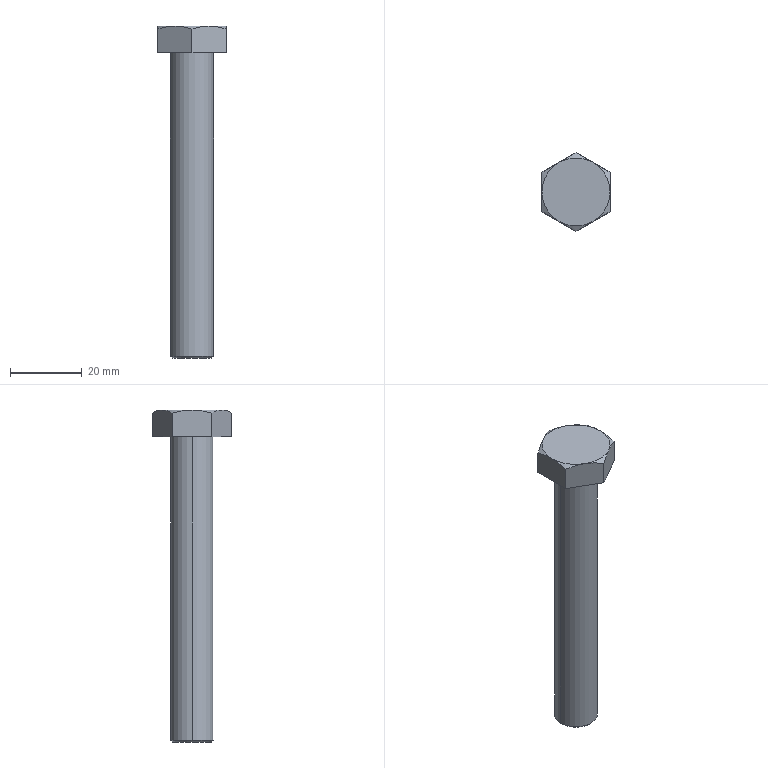Part | STEP file | M12-L85-0 | 1 solid | 19 faces | box 19 x 21.939 x 92.5 mm | volume 11946 mm3 | plane 9 | cone 8 | cylinder 2 | commonest cylinder face diameters 12 x2
STEP:
#1=CARTESIAN_POINT('',(-5.5,0.,-5.));
#2=VERTEX_POINT('',#1);
#3=CARTESIAN_POINT('',(5.5,0.,-5.));
#4=VERTEX_POINT('',#3);
#5=CARTESIAN_POINT('',(0.,0.,-5.));
#6=DIRECTION('',(0.,0.,-1.));
#7=DIRECTION('',(-1.,0.,0.));
#8=AXIS2_PLACEMENT_3D('',#5,#6,#7);
#9=CIRCLE('',#8,5.5);
#10=EDGE_CURVE('',#2,#4,#9,.T.);
#11=ORIENTED_EDGE('',*,*,#10,.F.);
#12=CARTESIAN_POINT('',(-6.,0.,-4.5));
#13=VERTEX_POINT('',#12);
#14=CARTESIAN_POINT('',(-5.5,0.,-5.));
#15=DIRECTION('',(-0.7071,0.,0.7071));
#16=VECTOR('',#15,1000.);
#17=LINE('',#14,#16);
#18=EDGE_CURVE('',#2,#13,#17,.T.);
#19=ORIENTED_EDGE('',*,*,#18,.T.);
#20=CARTESIAN_POINT('',(6.,0.,-4.5));
#21=VERTEX_POINT('',#20);
#22=CARTESIAN_POINT('',(0.,0.,-4.5));
#23=DIRECTION('',(0.,0.,1.));
#24=DIRECTION('',(-1.,0.,0.));
#25=AXIS2_PLACEMENT_3D('',#22,#23,#24);
#26=CIRCLE('',#25,6.);
#27=EDGE_CURVE('',#21,#13,#26,.T.);
#28=ORIENTED_EDGE('',*,*,#27,.F.);
#29=CARTESIAN_POINT('',(5.5,0.,-5.));
#30=DIRECTION('',(0.7071,0.,0.7071));
#31=VECTOR('',#30,1000.);
#32=LINE('',#29,#31);
#33=EDGE_CURVE('',#4,#21,#32,.T.);
#34=ORIENTED_EDGE('',*,*,#33,.F.);
#35=EDGE_LOOP('',(#11,#19,#28,#34));
#36=FACE_OUTER_BOUND('',#35,.T.);
#37=CARTESIAN_POINT('',(0.,0.,-5.));
#38=DIRECTION('',(0.,0.,1.));
#39=DIRECTION('',(1.,0.,0.));
#40=AXIS2_PLACEMENT_3D('',#37,#38,#39);
#41=CONICAL_SURFACE('',#40,5.5,0.7854);
#42=ADVANCED_FACE('',(#36),#41,.T.);
#43=ORIENTED_EDGE('',*,*,#27,.T.);
#44=CARTESIAN_POINT('',(-6.,0.,80.));
#45=VERTEX_POINT('',#44);
#46=CARTESIAN_POINT('',(-6.,0.,0.));
#47=DIRECTION('',(0.,0.,1.));
#48=VECTOR('',#47,1000.);
#49=LINE('',#46,#48);
#50=EDGE_CURVE('',#13,#45,#49,.T.);
#51=ORIENTED_EDGE('',*,*,#50,.T.);
#52=CARTESIAN_POINT('',(6.,0.,80.));
#53=VERTEX_POINT('',#52);
#54=CARTESIAN_POINT('',(0.,0.,80.));
#55=DIRECTION('',(0.,0.,-1.));
#56=DIRECTION('',(1.,0.,0.));
#57=AXIS2_PLACEMENT_3D('',#54,#55,#56);
#58=CIRCLE('',#57,6.);
#59=EDGE_CURVE('',#45,#53,#58,.T.);
#60=ORIENTED_EDGE('',*,*,#59,.T.);
#61=CARTESIAN_POINT('',(6.,0.,0.));
#62=DIRECTION('',(0.,0.,1.));
#63=VECTOR('',#62,1000.);
#64=LINE('',#61,#63);
#65=EDGE_CURVE('',#21,#53,#64,.T.);
#66=ORIENTED_EDGE('',*,*,#65,.F.);
#67=EDGE_LOOP('',(#43,#51,#60,#66));
#68=FACE_OUTER_BOUND('',#67,.T.);
#69=CARTESIAN_POINT('',(0.,0.,0.));
#70=DIRECTION('',(0.,0.,1.));
#71=DIRECTION('',(1.,0.,0.));
#72=AXIS2_PLACEMENT_3D('',#69,#70,#71);
#73=CYLINDRICAL_SURFACE('',#72,6.);
#74=ADVANCED_FACE('',(#68),#73,.T.);
#75=ORIENTED_EDGE('',*,*,#50,.F.);
#76=CARTESIAN_POINT('',(0.,0.,-4.5));
#77=DIRECTION('',(0.,0.,1.));
#78=DIRECTION('',(-1.,0.,0.));
#79=AXIS2_PLACEMENT_3D('',#76,#77,#78);
#80=CIRCLE('',#79,6.);
#81=EDGE_CURVE('',#13,#21,#80,.T.);
#82=ORIENTED_EDGE('',*,*,#81,.T.);
#83=ORIENTED_EDGE('',*,*,#65,.T.);
#84=CARTESIAN_POINT('',(0.,0.,80.));
#85=DIRECTION('',(0.,0.,-1.));
#86=DIRECTION('',(1.,0.,0.));
#87=AXIS2_PLACEMENT_3D('',#84,#85,#86);
#88=CIRCLE('',#87,6.);
#89=EDGE_CURVE('',#53,#45,#88,.T.);
#90=ORIENTED_EDGE('',*,*,#89,.T.);
#91=EDGE_LOOP('',(#75,#82,#83,#90));
#92=FACE_OUTER_BOUND('',#91,.T.);
#93=CARTESIAN_POINT('',(0.,0.,0.));
#94=DIRECTION('',(0.,0.,1.));
#95=DIRECTION('',(1.,0.,0.));
#96=AXIS2_PLACEMENT_3D('',#93,#94,#95);
#97=CYLINDRICAL_SURFACE('',#96,6.);
#98=ADVANCED_FACE('',(#92),#97,.T.);
#99=ORIENTED_EDGE('',*,*,#89,.F.);
#100=ORIENTED_EDGE('',*,*,#59,.F.);
#101=EDGE_LOOP('',(#99,#100));
#102=FACE_BOUND('',#101,.T.);
#103=CARTESIAN_POINT('',(9.5,-5.485,80.));
#104=VERTEX_POINT('',#103);
#105=CARTESIAN_POINT('',(9.5,5.485,80.));
#106=VERTEX_POINT('',#105);
#107=CARTESIAN_POINT('',(9.5,0.,80.));
#108=DIRECTION('',(0.,1.,0.));
#109=VECTOR('',#108,1000.);
#110=LINE('',#107,#109);
#111=EDGE_CURVE('',#104,#106,#110,.T.);
#112=ORIENTED_EDGE('',*,*,#111,.F.);
#113=CARTESIAN_POINT('',(0.,-10.97,80.));
#114=VERTEX_POINT('',#113);
#115=CARTESIAN_POINT('',(0.,-10.97,80.));
#116=DIRECTION('',(0.866,0.5,0.));
#117=VECTOR('',#116,1000.);
#118=LINE('',#115,#117);
#119=EDGE_CURVE('',#114,#104,#118,.T.);
#120=ORIENTED_EDGE('',*,*,#119,.F.);
#121=CARTESIAN_POINT('',(-9.5,-5.485,80.));
#122=VERTEX_POINT('',#121);
#123=CARTESIAN_POINT('',(-9.5,-5.485,80.));
#124=DIRECTION('',(0.866,-0.5,0.));
#125=VECTOR('',#124,1000.);
#126=LINE('',#123,#125);
#127=EDGE_CURVE('',#122,#114,#126,.T.);
#128=ORIENTED_EDGE('',*,*,#127,.F.);
#129=CARTESIAN_POINT('',(-9.5,5.485,80.));
#130=VERTEX_POINT('',#129);
#131=CARTESIAN_POINT('',(-9.5,0.,80.));
#132=DIRECTION('',(0.,-1.,0.));
#133=VECTOR('',#132,1000.);
#134=LINE('',#131,#133);
#135=EDGE_CURVE('',#130,#122,#134,.T.);
#136=ORIENTED_EDGE('',*,*,#135,.F.);
#137=CARTESIAN_POINT('',(0.,10.97,80.));
#138=VERTEX_POINT('',#137);
#139=CARTESIAN_POINT('',(0.,10.97,80.));
#140=DIRECTION('',(-0.866,-0.5,0.));
#141=VECTOR('',#140,1000.);
#142=LINE('',#139,#141);
#143=EDGE_CURVE('',#138,#130,#142,.T.);
#144=ORIENTED_EDGE('',*,*,#143,.F.);
#145=CARTESIAN_POINT('',(9.5,5.485,80.));
#146=DIRECTION('',(-0.866,0.5,0.));
#147=VECTOR('',#146,1000.);
#148=LINE('',#145,#147);
#149=EDGE_CURVE('',#106,#138,#148,.T.);
#150=ORIENTED_EDGE('',*,*,#149,.F.);
#151=EDGE_LOOP('',(#112,#120,#128,#136,#144,#150));
#152=FACE_OUTER_BOUND('',#151,.T.);
#153=CARTESIAN_POINT('',(0.,0.,80.));
#154=DIRECTION('',(0.,0.,1.));
#155=DIRECTION('',(1.,0.,0.));
#156=AXIS2_PLACEMENT_3D('',#153,#154,#155);
#157=PLANE('',#156);
#158=ADVANCED_FACE('',(#102,#152),#157,.F.);
#159=CARTESIAN_POINT('',(0.,10.97,86.651));
#160=VERTEX_POINT('',#159);
#161=CARTESIAN_POINT('',(4.75,8.227,87.5));
#162=VERTEX_POINT('',#161);
#163=CARTESIAN_POINT('',(0.,10.97,86.651));
#164=CARTESIAN_POINT('',(0.776,10.522,86.91));
#165=CARTESIAN_POINT('',(1.558,10.07,87.123));
#166=CARTESIAN_POINT('',(3.14,9.157,87.419));
#167=CARTESIAN_POINT('',(3.939,8.695,87.5));
#168=CARTESIAN_POINT('',(4.75,8.227,87.5));
#169=B_SPLINE_CURVE_WITH_KNOTS('',3,(#163,#164,#165,#166,#167,#168),.UNSPECIFIED.,.F.,.F.,(4,2,4),(0.,0.002775,0.00555),.UNSPECIFIED.);
#170=EDGE_CURVE('',#160,#162,#169,.T.);
#171=ORIENTED_EDGE('',*,*,#170,.T.);
#172=CARTESIAN_POINT('',(9.5,5.485,86.651));
#173=VERTEX_POINT('',#172);
#174=CARTESIAN_POINT('',(4.75,8.227,87.5));
#175=CARTESIAN_POINT('',(5.561,7.759,87.5));
#176=CARTESIAN_POINT('',(6.36,7.298,87.419));
#177=CARTESIAN_POINT('',(7.942,6.384,87.123));
#178=CARTESIAN_POINT('',(8.724,5.933,86.91));
#179=CARTESIAN_POINT('',(9.5,5.485,86.651));
#180=B_SPLINE_CURVE_WITH_KNOTS('',3,(#174,#175,#176,#177,#178,#179),.UNSPECIFIED.,.F.,.F.,(4,2,4),(0.,0.002775,0.00555),.UNSPECIFIED.);
#181=EDGE_CURVE('',#162,#173,#180,.T.);
#182=ORIENTED_EDGE('',*,*,#181,.T.);
#183=CARTESIAN_POINT('',(9.5,5.485,80.));
#184=DIRECTION('',(0.,0.,-1.));
#185=VECTOR('',#184,1000.);
#186=LINE('',#183,#185);
#187=EDGE_CURVE('',#173,#106,#186,.T.);
#188=ORIENTED_EDGE('',*,*,#187,.T.);
#189=ORIENTED_EDGE('',*,*,#149,.T.);
#190=CARTESIAN_POINT('',(0.,10.97,80.));
#191=DIRECTION('',(0.,0.,1.));
#192=VECTOR('',#191,1000.);
#193=LINE('',#190,#192);
#194=EDGE_CURVE('',#138,#160,#193,.T.);
#195=ORIENTED_EDGE('',*,*,#194,.T.);
#196=EDGE_LOOP('',(#171,#182,#188,#189,#195));
#197=FACE_OUTER_BOUND('',#196,.T.);
#198=CARTESIAN_POINT('',(9.5,5.485,80.));
#199=DIRECTION('',(0.5,0.866,0.));
#200=DIRECTION('',(-0.866,0.5,0.));
#201=AXIS2_PLACEMENT_3D('',#198,#199,#200);
#202=PLANE('',#201);
#203=ADVANCED_FACE('',(#197),#202,.T.);
#204=CARTESIAN_POINT('',(9.5,-0.000000001,87.5));
#205=VERTEX_POINT('',#204);
#206=CARTESIAN_POINT('',(9.5,5.485,86.651));
#207=CARTESIAN_POINT('',(9.5,4.589,86.91));
#208=CARTESIAN_POINT('',(9.5,3.686,87.123));
#209=CARTESIAN_POINT('',(9.5,1.859,87.419));
#210=CARTESIAN_POINT('',(9.5,0.936,87.5));
#211=CARTESIAN_POINT('',(9.5,-0.000000001,87.5));
#212=B_SPLINE_CURVE_WITH_KNOTS('',3,(#206,#207,#208,#209,#210,#211),.UNSPECIFIED.,.F.,.F.,(4,2,4),(0.,0.002775,0.00555),.UNSPECIFIED.);
#213=EDGE_CURVE('',#173,#205,#212,.T.);
#214=ORIENTED_EDGE('',*,*,#213,.T.);
#215=CARTESIAN_POINT('',(9.5,-5.485,86.651));
#216=VERTEX_POINT('',#215);
#217=CARTESIAN_POINT('',(9.5,-0.000000001,87.5));
#218=CARTESIAN_POINT('',(9.5,-0.936,87.5));
#219=CARTESIAN_POINT('',(9.5,-1.859,87.419));
#220=CARTESIAN_POINT('',(9.5,-3.686,87.123));
#221=CARTESIAN_POINT('',(9.5,-4.589,86.91));
#222=CARTESIAN_POINT('',(9.5,-5.485,86.651));
#223=B_SPLINE_CURVE_WITH_KNOTS('',3,(#217,#218,#219,#220,#221,#222),.UNSPECIFIED.,.F.,.F.,(4,2,4),(0.,0.002775,0.00555),.UNSPECIFIED.);
#224=EDGE_CURVE('',#205,#216,#223,.T.);
#225=ORIENTED_EDGE('',*,*,#224,.T.);
#226=CARTESIAN_POINT('',(9.5,-5.485,80.));
#227=DIRECTION('',(0.,0.,-1.));
#228=VECTOR('',#227,1000.);
#229=LINE('',#226,#228);
#230=EDGE_CURVE('',#216,#104,#229,.T.);
#231=ORIENTED_EDGE('',*,*,#230,.T.);
#232=ORIENTED_EDGE('',*,*,#111,.T.);
#233=ORIENTED_EDGE('',*,*,#187,.F.);
#234=EDGE_LOOP('',(#214,#225,#231,#232,#233));
#235=FACE_OUTER_BOUND('',#234,.T.);
#236=CARTESIAN_POINT('',(9.5,-5.485,80.));
#237=DIRECTION('',(1.,0.,0.));
#238=DIRECTION('',(0.,0.,-1.));
#239=AXIS2_PLACEMENT_3D('',#236,#237,#238);
#240=PLANE('',#239);
#241=ADVANCED_FACE('',(#235),#240,.T.);
#242=CARTESIAN_POINT('',(4.75,-8.227,87.5));
#243=VERTEX_POINT('',#242);
#244=CARTESIAN_POINT('',(9.5,-5.485,86.651));
#245=CARTESIAN_POINT('',(8.724,-5.933,86.91));
#246=CARTESIAN_POINT('',(7.942,-6.384,87.123));
#247=CARTESIAN_POINT('',(6.36,-7.298,87.419));
#248=CARTESIAN_POINT('',(5.561,-7.759,87.5));
#249=CARTESIAN_POINT('',(4.75,-8.227,87.5));
#250=B_SPLINE_CURVE_WITH_KNOTS('',3,(#244,#245,#246,#247,#248,#249),.UNSPECIFIED.,.F.,.F.,(4,2,4),(0.,0.002775,0.00555),.UNSPECIFIED.);
#251=EDGE_CURVE('',#216,#243,#250,.T.);
#252=ORIENTED_EDGE('',*,*,#251,.T.);
#253=CARTESIAN_POINT('',(0.,-10.97,86.651));
#254=VERTEX_POINT('',#253);
#255=CARTESIAN_POINT('',(4.75,-8.227,87.5));
#256=CARTESIAN_POINT('',(3.939,-8.695,87.5));
#257=CARTESIAN_POINT('',(3.14,-9.157,87.419));
#258=CARTESIAN_POINT('',(1.558,-10.07,87.123));
#259=CARTESIAN_POINT('',(0.776,-10.522,86.91));
#260=CARTESIAN_POINT('',(0.,-10.97,86.651));
#261=B_SPLINE_CURVE_WITH_KNOTS('',3,(#255,#256,#257,#258,#259,#260),.UNSPECIFIED.,.F.,.F.,(4,2,4),(0.,0.002775,0.00555),.UNSPECIFIED.);
#262=EDGE_CURVE('',#243,#254,#261,.T.);
#263=ORIENTED_EDGE('',*,*,#262,.T.);
#264=CARTESIAN_POINT('',(0.,-10.97,80.));
#265=DIRECTION('',(0.,0.,-1.));
#266=VECTOR('',#265,1000.);
#267=LINE('',#264,#266);
#268=EDGE_CURVE('',#254,#114,#267,.T.);
#269=ORIENTED_EDGE('',*,*,#268,.T.);
#270=ORIENTED_EDGE('',*,*,#119,.T.);
#271=ORIENTED_EDGE('',*,*,#230,.F.);
#272=EDGE_LOOP('',(#252,#263,#269,#270,#271));
#273=FACE_OUTER_BOUND('',#272,.T.);
#274=CARTESIAN_POINT('',(0.,-10.97,80.));
#275=DIRECTION('',(0.5,-0.866,0.));
#276=DIRECTION('',(0.866,0.5,0.));
#277=AXIS2_PLACEMENT_3D('',#274,#275,#276);
#278=PLANE('',#277);
#279=ADVANCED_FACE('',(#273),#278,.T.);
#280=CARTESIAN_POINT('',(-4.75,-8.227,87.5));
#281=VERTEX_POINT('',#280);
#282=CARTESIAN_POINT('',(0.,-10.97,86.651));
#283=CARTESIAN_POINT('',(-0.776,-10.522,86.91));
#284=CARTESIAN_POINT('',(-1.558,-10.07,87.123));
#285=CARTESIAN_POINT('',(-3.14,-9.157,87.419));
#286=CARTESIAN_POINT('',(-3.939,-8.695,87.5));
#287=CARTESIAN_POINT('',(-4.75,-8.227,87.5));
#288=B_SPLINE_CURVE_WITH_KNOTS('',3,(#282,#283,#284,#285,#286,#287),.UNSPECIFIED.,.F.,.F.,(4,2,4),(0.,0.002775,0.00555),.UNSPECIFIED.);
#289=EDGE_CURVE('',#254,#281,#288,.T.);
#290=ORIENTED_EDGE('',*,*,#289,.T.);
#291=CARTESIAN_POINT('',(-9.5,-5.485,86.651));
#292=VERTEX_POINT('',#291);
#293=CARTESIAN_POINT('',(-4.75,-8.227,87.5));
#294=CARTESIAN_POINT('',(-5.561,-7.759,87.5));
#295=CARTESIAN_POINT('',(-6.36,-7.298,87.419));
#296=CARTESIAN_POINT('',(-7.942,-6.384,87.123));
#297=CARTESIAN_POINT('',(-8.724,-5.933,86.91));
#298=CARTESIAN_POINT('',(-9.5,-5.485,86.651));
#299=B_SPLINE_CURVE_WITH_KNOTS('',3,(#293,#294,#295,#296,#297,#298),.UNSPECIFIED.,.F.,.F.,(4,2,4),(0.,0.002775,0.00555),.UNSPECIFIED.);
#300=EDGE_CURVE('',#281,#292,#299,.T.);
#301=ORIENTED_EDGE('',*,*,#300,.T.);
#302=CARTESIAN_POINT('',(-9.5,-5.485,80.));
#303=DIRECTION('',(0.,0.,-1.));
#304=VECTOR('',#303,1000.);
#305=LINE('',#302,#304);
#306=EDGE_CURVE('',#292,#122,#305,.T.);
#307=ORIENTED_EDGE('',*,*,#306,.T.);
#308=ORIENTED_EDGE('',*,*,#127,.T.);
#309=ORIENTED_EDGE('',*,*,#268,.F.);
#310=EDGE_LOOP('',(#290,#301,#307,#308,#309));
#311=FACE_OUTER_BOUND('',#310,.T.);
#312=CARTESIAN_POINT('',(-9.5,-5.485,80.));
#313=DIRECTION('',(-0.5,-0.866,0.));
#314=DIRECTION('',(0.866,-0.5,0.));
#315=AXIS2_PLACEMENT_3D('',#312,#313,#314);
#316=PLANE('',#315);
#317=ADVANCED_FACE('',(#311),#316,.T.);
#318=CARTESIAN_POINT('',(-9.5,0.,87.5));
#319=VERTEX_POINT('',#318);
#320=CARTESIAN_POINT('',(-9.5,-5.485,86.651));
#321=CARTESIAN_POINT('',(-9.5,-4.589,86.91));
#322=CARTESIAN_POINT('',(-9.5,-3.686,87.123));
#323=CARTESIAN_POINT('',(-9.5,-1.859,87.419));
#324=CARTESIAN_POINT('',(-9.5,-0.936,87.5));
#325=CARTESIAN_POINT('',(-9.5,0.,87.5));
#326=B_SPLINE_CURVE_WITH_KNOTS('',3,(#320,#321,#322,#323,#324,#325),.UNSPECIFIED.,.F.,.F.,(4,2,4),(0.,0.002775,0.00555),.UNSPECIFIED.);
#327=EDGE_CURVE('',#292,#319,#326,.T.);
#328=ORIENTED_EDGE('',*,*,#327,.T.);
#329=CARTESIAN_POINT('',(-9.5,5.485,86.651));
#330=VERTEX_POINT('',#329);
#331=CARTESIAN_POINT('',(-9.5,0.,87.5));
#332=CARTESIAN_POINT('',(-9.5,0.936,87.5));
#333=CARTESIAN_POINT('',(-9.5,1.859,87.419));
#334=CARTESIAN_POINT('',(-9.5,3.686,87.123));
#335=CARTESIAN_POINT('',(-9.5,4.589,86.91));
#336=CARTESIAN_POINT('',(-9.5,5.485,86.651));
#337=B_SPLINE_CURVE_WITH_KNOTS('',3,(#331,#332,#333,#334,#335,#336),.UNSPECIFIED.,.F.,.F.,(4,2,4),(0.,0.002775,0.00555),.UNSPECIFIED.);
#338=EDGE_CURVE('',#319,#330,#337,.T.);
#339=ORIENTED_EDGE('',*,*,#338,.T.);
#340=CARTESIAN_POINT('',(-9.5,5.485,80.));
#341=DIRECTION('',(0.,0.,-1.));
#342=VECTOR('',#341,1000.);
#343=LINE('',#340,#342);
#344=EDGE_CURVE('',#330,#130,#343,.T.);
#345=ORIENTED_EDGE('',*,*,#344,.T.);
#346=ORIENTED_EDGE('',*,*,#135,.T.);
#347=ORIENTED_EDGE('',*,*,#306,.F.);
#348=EDGE_LOOP('',(#328,#339,#345,#346,#347));
#349=FACE_OUTER_BOUND('',#348,.T.);
#350=CARTESIAN_POINT('',(-9.5,5.485,80.));
#351=DIRECTION('',(-1.,0.,0.));
#352=DIRECTION('',(0.,0.,1.));
#353=AXIS2_PLACEMENT_3D('',#350,#351,#352);
#354=PLANE('',#353);
#355=ADVANCED_FACE('',(#349),#354,.T.);
#356=CARTESIAN_POINT('',(-4.75,8.227,87.5));
#357=VERTEX_POINT('',#356);
#358=CARTESIAN_POINT('',(-9.5,5.485,86.651));
#359=CARTESIAN_POINT('',(-8.724,5.933,86.91));
#360=CARTESIAN_POINT('',(-7.942,6.384,87.123));
#361=CARTESIAN_POINT('',(-6.36,7.298,87.419));
#362=CARTESIAN_POINT('',(-5.561,7.759,87.5));
#363=CARTESIAN_POINT('',(-4.75,8.227,87.5));
#364=B_SPLINE_CURVE_WITH_KNOTS('',3,(#358,#359,#360,#361,#362,#363),.UNSPECIFIED.,.F.,.F.,(4,2,4),(0.,0.002775,0.00555),.UNSPECIFIED.);
#365=EDGE_CURVE('',#330,#357,#364,.T.);
#366=ORIENTED_EDGE('',*,*,#365,.T.);
#367=CARTESIAN_POINT('',(-4.75,8.227,87.5));
#368=CARTESIAN_POINT('',(-3.939,8.695,87.5));
#369=CARTESIAN_POINT('',(-3.14,9.157,87.419));
#370=CARTESIAN_POINT('',(-1.558,10.07,87.123));
#371=CARTESIAN_POINT('',(-0.776,10.522,86.91));
#372=CARTESIAN_POINT('',(0.,10.97,86.651));
#373=B_SPLINE_CURVE_WITH_KNOTS('',3,(#367,#368,#369,#370,#371,#372),.UNSPECIFIED.,.F.,.F.,(4,2,4),(0.,0.002775,0.00555),.UNSPECIFIED.);
#374=EDGE_CURVE('',#357,#160,#373,.T.);
#375=ORIENTED_EDGE('',*,*,#374,.T.);
#376=ORIENTED_EDGE('',*,*,#194,.F.);
#377=ORIENTED_EDGE('',*,*,#143,.T.);
#378=ORIENTED_EDGE('',*,*,#344,.F.);
#379=EDGE_LOOP('',(#366,#375,#376,#377,#378));
#380=FACE_OUTER_BOUND('',#379,.T.);
#381=CARTESIAN_POINT('',(0.,10.97,80.));
#382=DIRECTION('',(-0.5,0.866,0.));
#383=DIRECTION('',(-0.866,-0.5,0.));
#384=AXIS2_PLACEMENT_3D('',#381,#382,#383);
#385=PLANE('',#384);
#386=ADVANCED_FACE('',(#380),#385,.T.);
#387=ORIENTED_EDGE('',*,*,#181,.F.);
#388=CARTESIAN_POINT('',(0.,0.,87.5));
#389=DIRECTION('',(0.,0.,-1.));
#390=DIRECTION('',(-1.,0.,0.));
#391=AXIS2_PLACEMENT_3D('',#388,#389,#390);
#392=CIRCLE('',#391,9.5);
#393=EDGE_CURVE('',#162,#205,#392,.T.);
#394=ORIENTED_EDGE('',*,*,#393,.T.);
#395=ORIENTED_EDGE('',*,*,#213,.F.);
#396=EDGE_LOOP('',(#387,#394,#395));
#397=FACE_OUTER_BOUND('',#396,.T.);
#398=CARTESIAN_POINT('',(0.,0.,86.646));
#399=DIRECTION('',(0.,0.,-1.));
#400=DIRECTION('',(-1.,0.,0.));
#401=AXIS2_PLACEMENT_3D('',#398,#399,#400);
#402=CONICAL_SURFACE('',#401,10.978,1.047);
#403=ADVANCED_FACE('',(#397),#402,.T.);
#404=ORIENTED_EDGE('',*,*,#374,.F.);
#405=CARTESIAN_POINT('',(0.,0.,87.5));
#406=DIRECTION('',(0.,0.,-1.));
#407=DIRECTION('',(-1.,0.,0.));
#408=AXIS2_PLACEMENT_3D('',#405,#406,#407);
#409=CIRCLE('',#408,9.5);
#410=EDGE_CURVE('',#357,#162,#409,.T.);
#411=ORIENTED_EDGE('',*,*,#410,.T.);
#412=ORIENTED_EDGE('',*,*,#170,.F.);
#413=EDGE_LOOP('',(#404,#411,#412));
#414=FACE_OUTER_BOUND('',#413,.T.);
#415=CARTESIAN_POINT('',(0.,0.,86.646));
#416=DIRECTION('',(0.,0.,-1.));
#417=DIRECTION('',(-1.,0.,0.));
#418=AXIS2_PLACEMENT_3D('',#415,#416,#417);
#419=CONICAL_SURFACE('',#418,10.978,1.047);
#420=ADVANCED_FACE('',(#414),#419,.T.);
#421=ORIENTED_EDGE('',*,*,#224,.F.);
#422=CARTESIAN_POINT('',(0.,0.,87.5));
#423=DIRECTION('',(0.,0.,-1.));
#424=DIRECTION('',(-1.,0.,0.));
#425=AXIS2_PLACEMENT_3D('',#422,#423,#424);
#426=CIRCLE('',#425,9.5);
#427=EDGE_CURVE('',#205,#243,#426,.T.);
#428=ORIENTED_EDGE('',*,*,#427,.T.);
#429=ORIENTED_EDGE('',*,*,#251,.F.);
#430=EDGE_LOOP('',(#421,#428,#429));
#431=FACE_OUTER_BOUND('',#430,.T.);
#432=CARTESIAN_POINT('',(0.,0.,86.646));
#433=DIRECTION('',(0.,0.,-1.));
#434=DIRECTION('',(-1.,0.,0.));
#435=AXIS2_PLACEMENT_3D('',#432,#433,#434);
#436=CONICAL_SURFACE('',#435,10.978,1.047);
#437=ADVANCED_FACE('',(#431),#436,.T.);
#438=ORIENTED_EDGE('',*,*,#262,.F.);
#439=CARTESIAN_POINT('',(0.,0.,87.5));
#440=DIRECTION('',(0.,0.,-1.));
#441=DIRECTION('',(-1.,0.,0.));
#442=AXIS2_PLACEMENT_3D('',#439,#440,#441);
#443=CIRCLE('',#442,9.5);
#444=EDGE_CURVE('',#243,#281,#443,.T.);
#445=ORIENTED_EDGE('',*,*,#444,.T.);
#446=ORIENTED_EDGE('',*,*,#289,.F.);
#447=EDGE_LOOP('',(#438,#445,#446));
#448=FACE_OUTER_BOUND('',#447,.T.);
#449=CARTESIAN_POINT('',(0.,0.,86.646));
#450=DIRECTION('',(0.,0.,-1.));
#451=DIRECTION('',(-1.,0.,0.));
#452=AXIS2_PLACEMENT_3D('',#449,#450,#451);
#453=CONICAL_SURFACE('',#452,10.978,1.047);
#454=ADVANCED_FACE('',(#448),#453,.T.);
#455=ORIENTED_EDGE('',*,*,#300,.F.);
#456=CARTESIAN_POINT('',(0.,0.,87.5));
#457=DIRECTION('',(0.,0.,-1.));
#458=DIRECTION('',(-1.,0.,0.));
#459=AXIS2_PLACEMENT_3D('',#456,#457,#458);
#460=CIRCLE('',#459,9.5);
#461=EDGE_CURVE('',#281,#319,#460,.T.);
#462=ORIENTED_EDGE('',*,*,#461,.T.);
#463=ORIENTED_EDGE('',*,*,#327,.F.);
#464=EDGE_LOOP('',(#455,#462,#463));
#465=FACE_OUTER_BOUND('',#464,.T.);
#466=CARTESIAN_POINT('',(0.,0.,86.646));
#467=DIRECTION('',(0.,0.,-1.));
#468=DIRECTION('',(-1.,0.,0.));
#469=AXIS2_PLACEMENT_3D('',#466,#467,#468);
#470=CONICAL_SURFACE('',#469,10.978,1.047);
#471=ADVANCED_FACE('',(#465),#470,.T.);
#472=ORIENTED_EDGE('',*,*,#338,.F.);
#473=CARTESIAN_POINT('',(0.,0.,87.5));
#474=DIRECTION('',(0.,0.,-1.));
#475=DIRECTION('',(-1.,0.,0.));
#476=AXIS2_PLACEMENT_3D('',#473,#474,#475);
#477=CIRCLE('',#476,9.5);
#478=EDGE_CURVE('',#319,#357,#477,.T.);
#479=ORIENTED_EDGE('',*,*,#478,.T.);
#480=ORIENTED_EDGE('',*,*,#365,.F.);
#481=EDGE_LOOP('',(#472,#479,#480));
#482=FACE_OUTER_BOUND('',#481,.T.);
#483=CARTESIAN_POINT('',(0.,0.,86.646));
#484=DIRECTION('',(0.,0.,-1.));
#485=DIRECTION('',(-1.,0.,0.));
#486=AXIS2_PLACEMENT_3D('',#483,#484,#485);
#487=CONICAL_SURFACE('',#486,10.978,1.047);
#488=ADVANCED_FACE('',(#482),#487,.T.);
#489=ORIENTED_EDGE('',*,*,#461,.F.);
#490=ORIENTED_EDGE('',*,*,#444,.F.);
#491=ORIENTED_EDGE('',*,*,#427,.F.);
#492=ORIENTED_EDGE('',*,*,#393,.F.);
#493=ORIENTED_EDGE('',*,*,#410,.F.);
#494=ORIENTED_EDGE('',*,*,#478,.F.);
#495=EDGE_LOOP('',(#489,#490,#491,#492,#493,#494));
#496=FACE_OUTER_BOUND('',#495,.T.);
#497=CARTESIAN_POINT('',(0.,0.,87.5));
#498=DIRECTION('',(0.,0.,1.));
#499=DIRECTION('',(1.,0.,0.));
#500=AXIS2_PLACEMENT_3D('',#497,#498,#499);
#501=PLANE('',#500);
#502=ADVANCED_FACE('',(#496),#501,.T.);
#503=CARTESIAN_POINT('',(0.,0.,-5.));
#504=DIRECTION('',(0.,0.,-1.));
#505=DIRECTION('',(-1.,0.,0.));
#506=AXIS2_PLACEMENT_3D('',#503,#504,#505);
#507=CIRCLE('',#506,5.5);
#508=EDGE_CURVE('',#4,#2,#507,.T.);
#509=ORIENTED_EDGE('',*,*,#508,.T.);
#510=ORIENTED_EDGE('',*,*,#10,.T.);
#511=EDGE_LOOP('',(#509,#510));
#512=FACE_OUTER_BOUND('',#511,.T.);
#513=CARTESIAN_POINT('',(0.,0.,-5.));
#514=DIRECTION('',(0.,0.,-1.));
#515=DIRECTION('',(-1.,0.,0.));
#516=AXIS2_PLACEMENT_3D('',#513,#514,#515);
#517=PLANE('',#516);
#518=ADVANCED_FACE('',(#512),#517,.T.);
#519=ORIENTED_EDGE('',*,*,#18,.F.);
#520=ORIENTED_EDGE('',*,*,#508,.F.);
#521=ORIENTED_EDGE('',*,*,#33,.T.);
#522=ORIENTED_EDGE('',*,*,#81,.F.);
#523=EDGE_LOOP('',(#519,#520,#521,#522));
#524=FACE_OUTER_BOUND('',#523,.T.);
#525=CARTESIAN_POINT('',(0.,0.,-5.));
#526=DIRECTION('',(0.,0.,1.));
#527=DIRECTION('',(1.,0.,0.));
#528=AXIS2_PLACEMENT_3D('',#525,#526,#527);
#529=CONICAL_SURFACE('',#528,5.5,0.7854);
#530=ADVANCED_FACE('',(#524),#529,.T.);
#531=CLOSED_SHELL('',(#42,#74,#98,#158,#203,#241,#279,#317,#355,#386,#403,#420,#437,#454,#471,#488,#502,#518,#530));
#532=MANIFOLD_SOLID_BREP('',#531);
#533=CARTESIAN_POINT('',(0.,0.,0.));
#534=DIRECTION('',(0.,0.,1.));
#535=DIRECTION('',(1.,0.,0.));
#536=AXIS2_PLACEMENT_3D('',#533,#534,#535);
#537=(LENGTH_UNIT()NAMED_UNIT(*)SI_UNIT(.MILLI.,.METRE.));
#538=UNCERTAINTY_MEASURE_WITH_UNIT(LENGTH_MEASURE(0.00001),#537,'','');
#539=(NAMED_UNIT(*)PLANE_ANGLE_UNIT()SI_UNIT($,.RADIAN.));
#540=(NAMED_UNIT(*)SI_UNIT($,.STERADIAN.)SOLID_ANGLE_UNIT());
#541=(GEOMETRIC_REPRESENTATION_CONTEXT(3)GLOBAL_UNCERTAINTY_ASSIGNED_CONTEXT((#538))GLOBAL_UNIT_ASSIGNED_CONTEXT((#537,#539,#540))REPRESENTATION_CONTEXT('',''));
#542=ADVANCED_BREP_SHAPE_REPRESENTATION('',(#532,#536),#541);